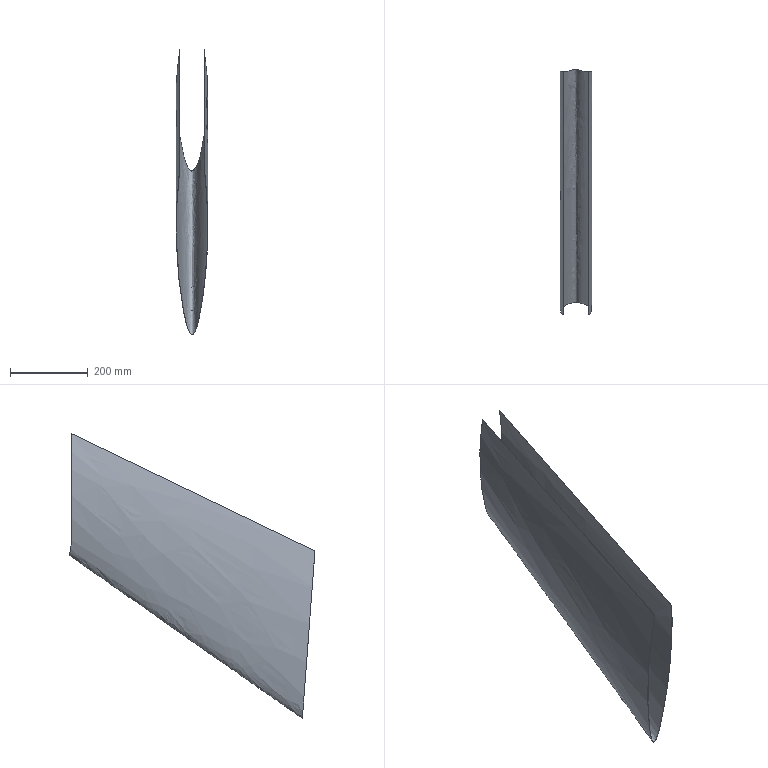Part | SolidWorks | features BaseBody 1 | 1 solid | 10 faces | box 81.981 x 634.565 x 735.208 mm | volume 421201 mm3 | spline 6 | plane 2 | cylinder 2 | commonest cylinder face diameters 224.558 x2